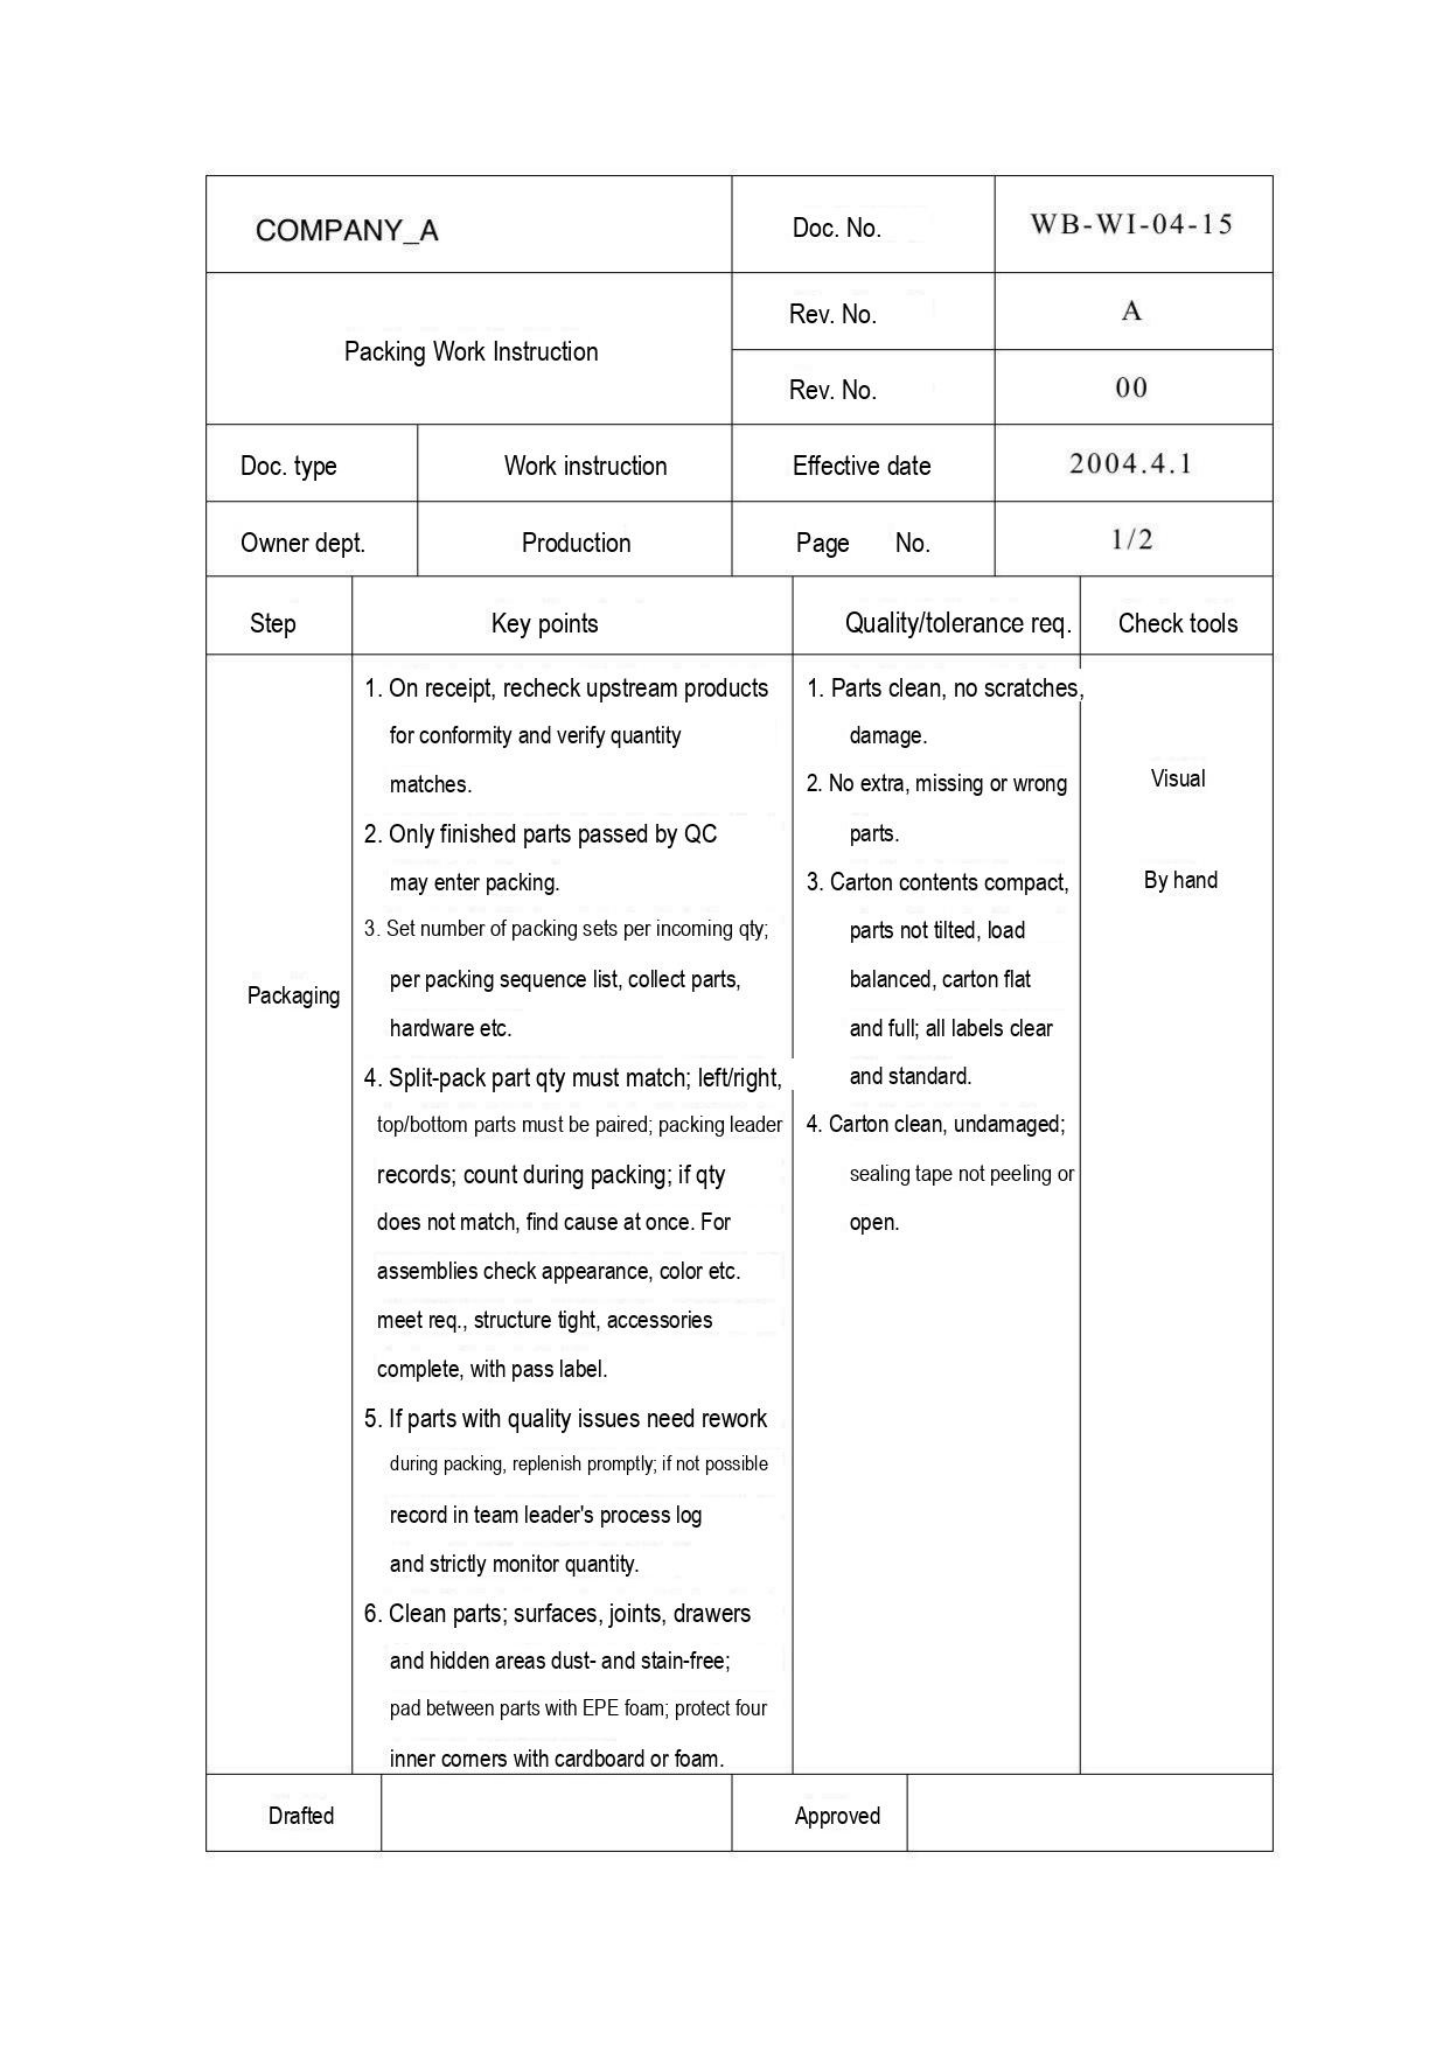| COMPANY_A | | Doc. No. | WB-WI-04-15 |
|---|---|---|---|
| Packing Work Instruction | | Rev. No. | A |
| | | Rev. No. | 00 |
| Doc. type | Work instruction | Effective date | 2004.4.1 |
| Owner dept. | Production | Page No. | 1/2 |

| Step | Key points | Quality/tolerance req. | Check tools |
|---|---|---|---|
| Packaging | 1. On receipt, recheck upstream products for conformity and verify quantity matches.<br>2. Only finished parts passed by QC may enter packing.<br>3. Set number of packing sets per incoming qty; per packing sequence list, collect parts, hardware etc.<br>4. Split-pack part qty must match; left/right, top/bottom parts must be paired; packing leader records; count during packing; if qty does not match, find cause at once. For assemblies check appearance, color etc. meet req., structure tight, accessories complete, with pass label.<br>5. If parts with quality issues need rework during packing, replenish promptly; if not possible record in team leader's process log and strictly monitor quantity.<br>6. Clean parts; surfaces, joints, drawers and hidden areas dust- and stain-free; pad between parts with EPE foam; protect four inner corners with cardboard or foam. | 1. Parts clean, no scratches, damage.<br>2. No extra, missing or wrong parts.<br>3. Carton contents compact, parts not tilted, load balanced, carton flat and full; all labels clear and standard.<br>4. Carton clean, undamaged; sealing tape not peeling or open. | Visual<br><br>By hand |

| Drafted | | Approved | |
|---|---|---|---|
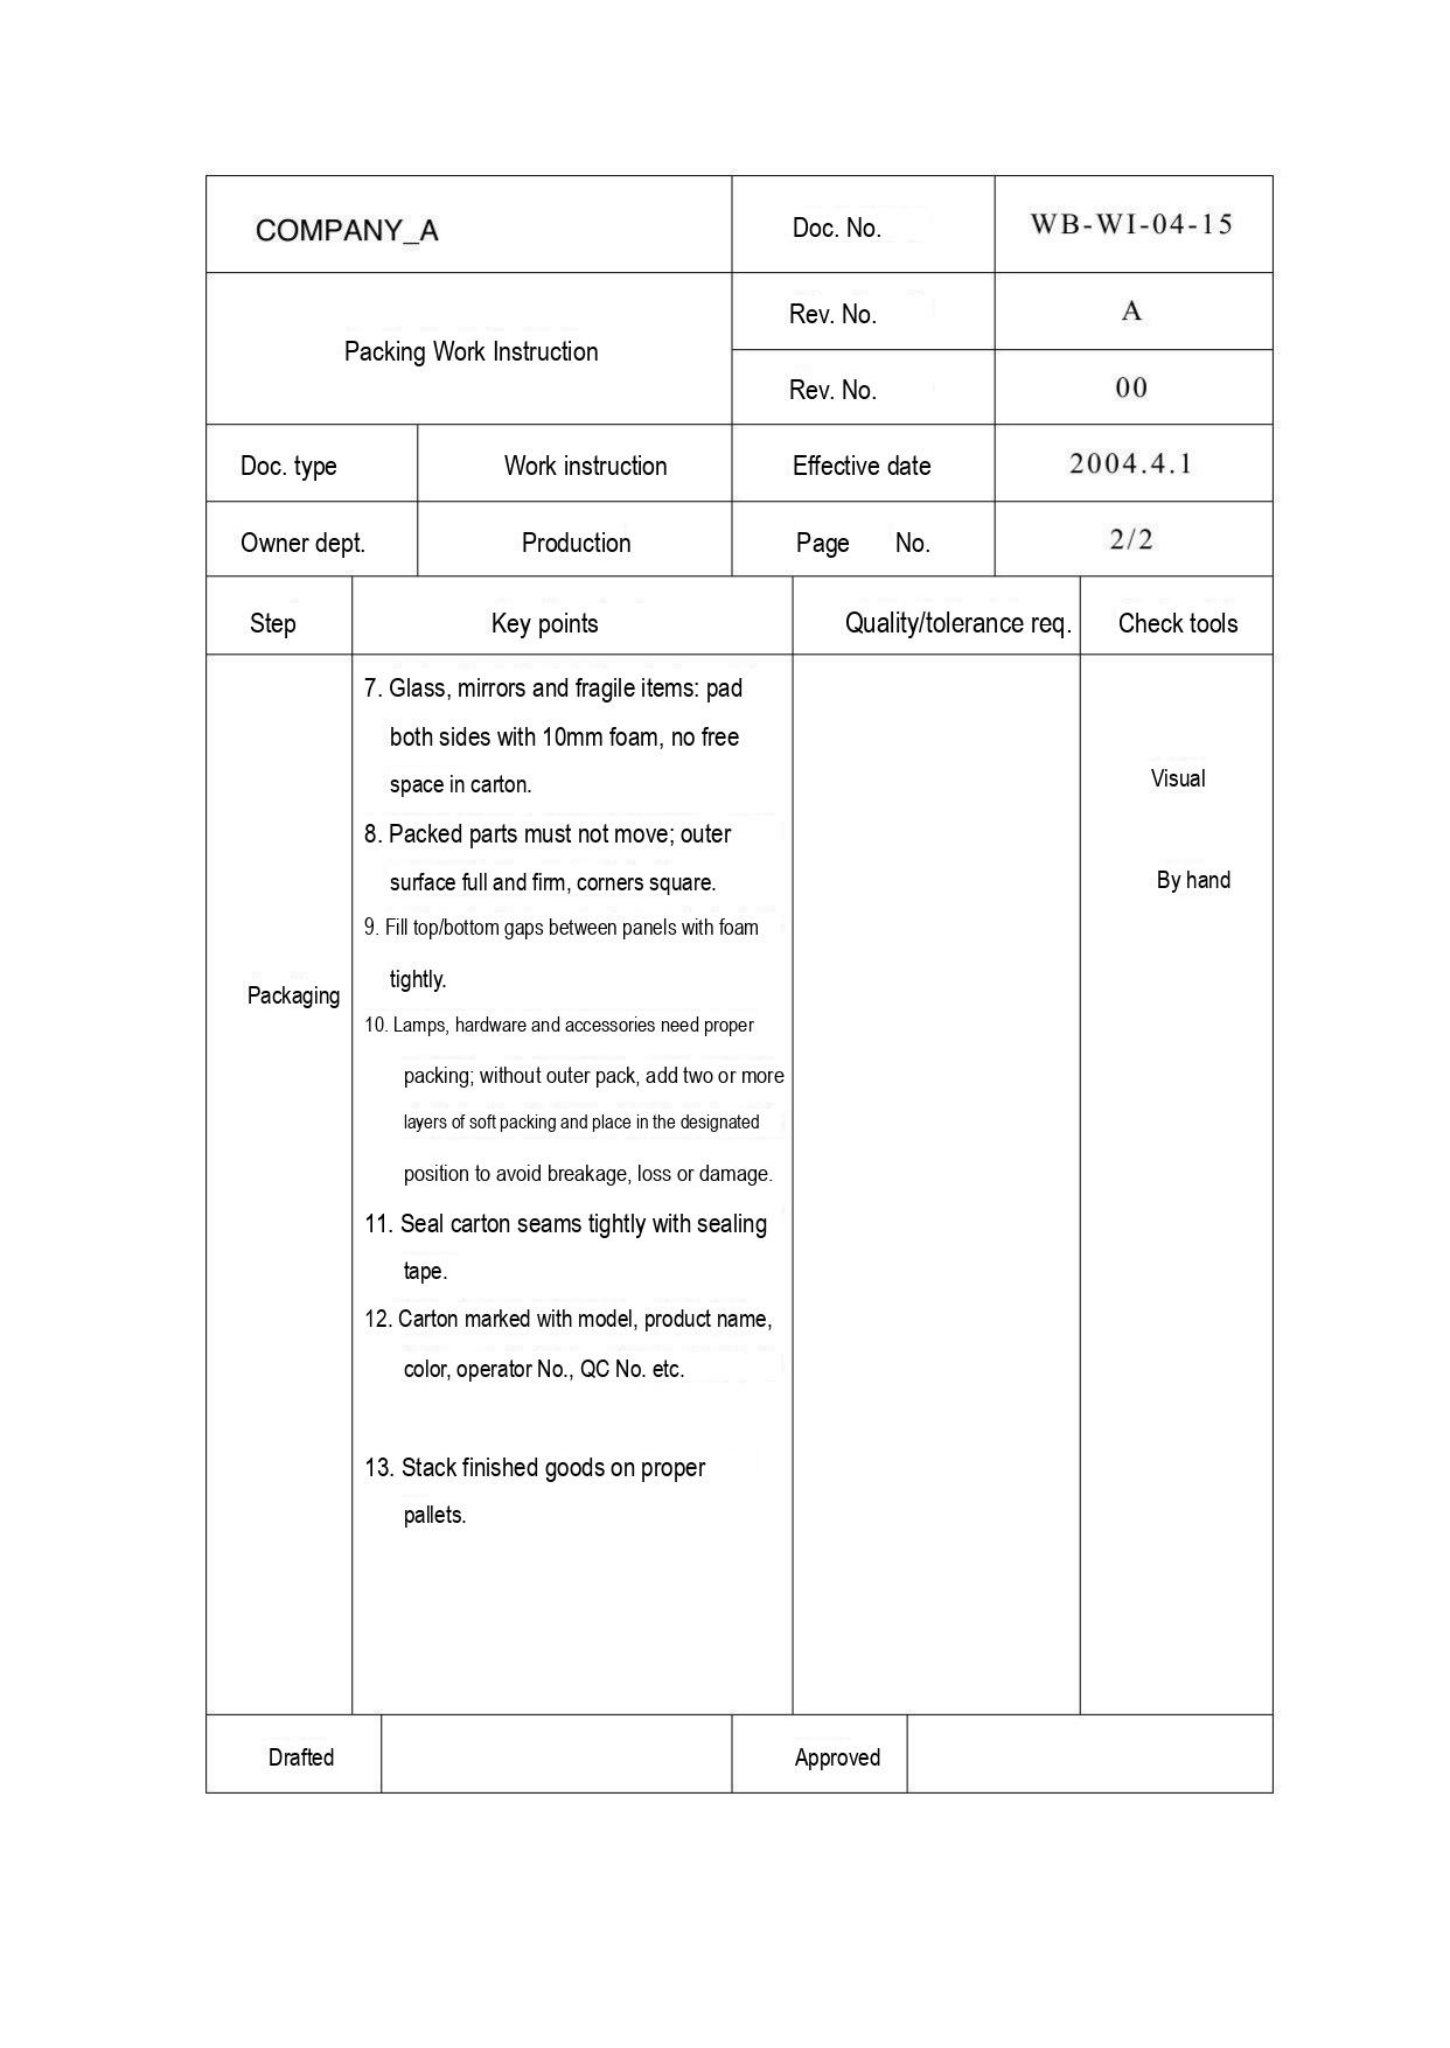| COMPANY_A | | Doc. No. | WB-WI-04-15 |
|---|---|---|---|
| Packing Work Instruction | | Rev. No. | A |
| | | Rev. No. | 00 |
| Doc. type | Work instruction | Effective date | 2004.4.1 |
| Owner dept. | Production | Page No. | 2/2 |

| Step | Key points | Quality/tolerance req. | Check tools |
|---|---|---|---|
| Packaging | 7. Glass, mirrors and fragile items: pad both sides with 10mm foam, no free space in carton.<br>8. Packed parts must not move; outer surface full and firm, corners square.<br>9. Fill top/bottom gaps between panels with foam tightly.<br>10. Lamps, hardware and accessories need proper packing; without outer pack, add two or more layers of soft packing and place in the designated position to avoid breakage, loss or damage.<br>11. Seal carton seams tightly with sealing tape.<br>12. Carton marked with model, product name, color, operator No., QC No. etc.<br>13. Stack finished goods on proper pallets. | | Visual<br>By hand |

| Drafted | | Approved | |
|---|---|---|---|